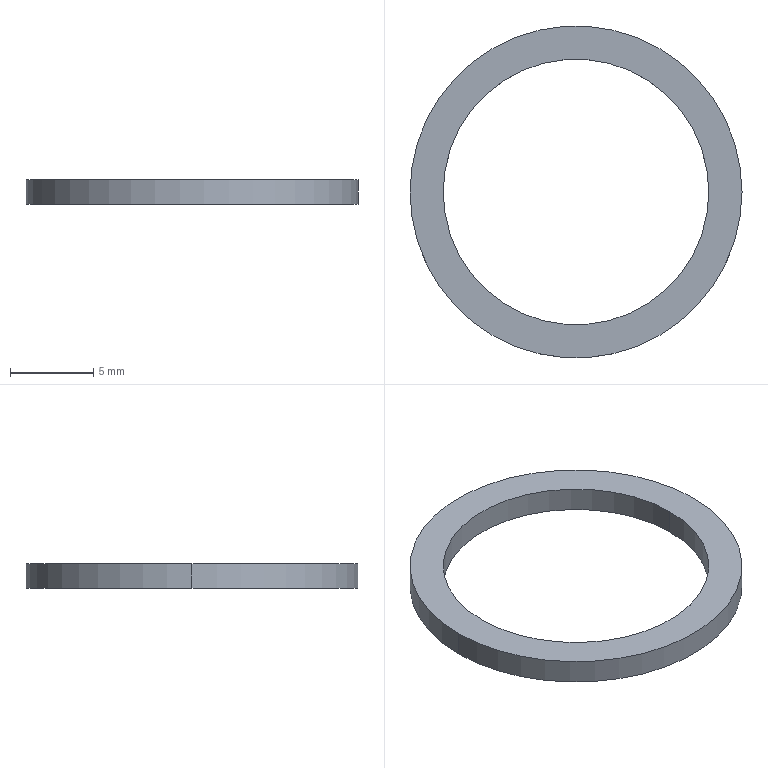Part | SolidWorks | features Extrusion 1 | 1 solid | 6 faces | box 20 x 20 x 1.5 mm | volume 169.646 mm3 | cylinder 4 | plane 2 | commonest cylinder face diameters 16 x2 20 x2
STEP:
#1=CARTESIAN_POINT('',(-8.,0.,1.5));
#2=VERTEX_POINT('',#1);
#3=CARTESIAN_POINT('',(8.,0.,1.5));
#4=VERTEX_POINT('',#3);
#5=CARTESIAN_POINT('',(0.,0.,1.5));
#6=DIRECTION('',(0.,0.,1.));
#7=DIRECTION('',(1.,0.,0.));
#8=AXIS2_PLACEMENT_3D('',#5,#6,#7);
#9=CIRCLE('',#8,8.);
#10=EDGE_CURVE('',#2,#4,#9,.T.);
#11=ORIENTED_EDGE('',*,*,#10,.T.);
#12=CARTESIAN_POINT('',(8.,0.,0.));
#13=VERTEX_POINT('',#12);
#14=CARTESIAN_POINT('',(8.,0.,1.5));
#15=DIRECTION('',(0.,0.,-1.));
#16=VECTOR('',#15,1000.);
#17=LINE('',#14,#16);
#18=EDGE_CURVE('',#4,#13,#17,.T.);
#19=ORIENTED_EDGE('',*,*,#18,.T.);
#20=CARTESIAN_POINT('',(-8.,0.,0.));
#21=VERTEX_POINT('',#20);
#22=CARTESIAN_POINT('',(0.,0.,0.));
#23=DIRECTION('',(0.,0.,1.));
#24=DIRECTION('',(1.,0.,0.));
#25=AXIS2_PLACEMENT_3D('',#22,#23,#24);
#26=CIRCLE('',#25,8.);
#27=EDGE_CURVE('',#21,#13,#26,.T.);
#28=ORIENTED_EDGE('',*,*,#27,.F.);
#29=CARTESIAN_POINT('',(-8.,0.,1.5));
#30=DIRECTION('',(0.,0.,-1.));
#31=VECTOR('',#30,1000.);
#32=LINE('',#29,#31);
#33=EDGE_CURVE('',#2,#21,#32,.T.);
#34=ORIENTED_EDGE('',*,*,#33,.F.);
#35=EDGE_LOOP('',(#11,#19,#28,#34));
#36=FACE_OUTER_BOUND('',#35,.T.);
#37=CARTESIAN_POINT('',(0.,0.,1.5));
#38=DIRECTION('',(0.,0.,-1.));
#39=DIRECTION('',(-1.,0.,0.));
#40=AXIS2_PLACEMENT_3D('',#37,#38,#39);
#41=CYLINDRICAL_SURFACE('',#40,8.);
#42=ADVANCED_FACE('',(#36),#41,.F.);
#43=CARTESIAN_POINT('',(10.,0.,1.5));
#44=VERTEX_POINT('',#43);
#45=CARTESIAN_POINT('',(-10.,0.,1.5));
#46=VERTEX_POINT('',#45);
#47=CARTESIAN_POINT('',(0.,0.,1.5));
#48=DIRECTION('',(0.,0.,1.));
#49=DIRECTION('',(1.,0.,0.));
#50=AXIS2_PLACEMENT_3D('',#47,#48,#49);
#51=CIRCLE('',#50,10.);
#52=EDGE_CURVE('',#44,#46,#51,.T.);
#53=ORIENTED_EDGE('',*,*,#52,.F.);
#54=CARTESIAN_POINT('',(10.,0.,0.));
#55=VERTEX_POINT('',#54);
#56=CARTESIAN_POINT('',(10.,0.,1.5));
#57=DIRECTION('',(0.,0.,-1.));
#58=VECTOR('',#57,1000.);
#59=LINE('',#56,#58);
#60=EDGE_CURVE('',#44,#55,#59,.T.);
#61=ORIENTED_EDGE('',*,*,#60,.T.);
#62=CARTESIAN_POINT('',(-10.,0.,0.));
#63=VERTEX_POINT('',#62);
#64=CARTESIAN_POINT('',(0.,0.,0.));
#65=DIRECTION('',(0.,0.,1.));
#66=DIRECTION('',(1.,0.,0.));
#67=AXIS2_PLACEMENT_3D('',#64,#65,#66);
#68=CIRCLE('',#67,10.);
#69=EDGE_CURVE('',#55,#63,#68,.T.);
#70=ORIENTED_EDGE('',*,*,#69,.T.);
#71=CARTESIAN_POINT('',(-10.,0.,1.5));
#72=DIRECTION('',(0.,0.,-1.));
#73=VECTOR('',#72,1000.);
#74=LINE('',#71,#73);
#75=EDGE_CURVE('',#46,#63,#74,.T.);
#76=ORIENTED_EDGE('',*,*,#75,.F.);
#77=EDGE_LOOP('',(#53,#61,#70,#76));
#78=FACE_OUTER_BOUND('',#77,.T.);
#79=CARTESIAN_POINT('',(0.,0.,1.5));
#80=DIRECTION('',(0.,0.,-1.));
#81=DIRECTION('',(-1.,0.,0.));
#82=AXIS2_PLACEMENT_3D('',#79,#80,#81);
#83=CYLINDRICAL_SURFACE('',#82,10.);
#84=ADVANCED_FACE('',(#78),#83,.T.);
#85=CARTESIAN_POINT('',(0.,0.,1.5));
#86=DIRECTION('',(0.,0.,1.));
#87=DIRECTION('',(1.,0.,0.));
#88=AXIS2_PLACEMENT_3D('',#85,#86,#87);
#89=CIRCLE('',#88,10.);
#90=EDGE_CURVE('',#46,#44,#89,.T.);
#91=ORIENTED_EDGE('',*,*,#90,.T.);
#92=ORIENTED_EDGE('',*,*,#52,.T.);
#93=EDGE_LOOP('',(#91,#92));
#94=FACE_OUTER_BOUND('',#93,.T.);
#95=ORIENTED_EDGE('',*,*,#10,.F.);
#96=CARTESIAN_POINT('',(0.,0.,1.5));
#97=DIRECTION('',(0.,0.,1.));
#98=DIRECTION('',(1.,0.,0.));
#99=AXIS2_PLACEMENT_3D('',#96,#97,#98);
#100=CIRCLE('',#99,8.);
#101=EDGE_CURVE('',#4,#2,#100,.T.);
#102=ORIENTED_EDGE('',*,*,#101,.F.);
#103=EDGE_LOOP('',(#95,#102));
#104=FACE_BOUND('',#103,.T.);
#105=CARTESIAN_POINT('',(0.,0.,1.5));
#106=DIRECTION('',(0.,0.,1.));
#107=DIRECTION('',(1.,0.,0.));
#108=AXIS2_PLACEMENT_3D('',#105,#106,#107);
#109=PLANE('',#108);
#110=ADVANCED_FACE('',(#94,#104),#109,.T.);
#111=CARTESIAN_POINT('',(0.,0.,0.));
#112=DIRECTION('',(0.,0.,1.));
#113=DIRECTION('',(1.,0.,0.));
#114=AXIS2_PLACEMENT_3D('',#111,#112,#113);
#115=CIRCLE('',#114,10.);
#116=EDGE_CURVE('',#63,#55,#115,.T.);
#117=ORIENTED_EDGE('',*,*,#116,.F.);
#118=ORIENTED_EDGE('',*,*,#69,.F.);
#119=EDGE_LOOP('',(#117,#118));
#120=FACE_OUTER_BOUND('',#119,.T.);
#121=ORIENTED_EDGE('',*,*,#27,.T.);
#122=CARTESIAN_POINT('',(0.,0.,0.));
#123=DIRECTION('',(0.,0.,1.));
#124=DIRECTION('',(1.,0.,0.));
#125=AXIS2_PLACEMENT_3D('',#122,#123,#124);
#126=CIRCLE('',#125,8.);
#127=EDGE_CURVE('',#13,#21,#126,.T.);
#128=ORIENTED_EDGE('',*,*,#127,.T.);
#129=EDGE_LOOP('',(#121,#128));
#130=FACE_BOUND('',#129,.T.);
#131=CARTESIAN_POINT('',(0.,0.,0.));
#132=DIRECTION('',(0.,0.,1.));
#133=DIRECTION('',(1.,0.,0.));
#134=AXIS2_PLACEMENT_3D('',#131,#132,#133);
#135=PLANE('',#134);
#136=ADVANCED_FACE('',(#120,#130),#135,.F.);
#137=ORIENTED_EDGE('',*,*,#60,.F.);
#138=ORIENTED_EDGE('',*,*,#90,.F.);
#139=ORIENTED_EDGE('',*,*,#75,.T.);
#140=ORIENTED_EDGE('',*,*,#116,.T.);
#141=EDGE_LOOP('',(#137,#138,#139,#140));
#142=FACE_OUTER_BOUND('',#141,.T.);
#143=CARTESIAN_POINT('',(0.,0.,1.5));
#144=DIRECTION('',(0.,0.,-1.));
#145=DIRECTION('',(-1.,0.,0.));
#146=AXIS2_PLACEMENT_3D('',#143,#144,#145);
#147=CYLINDRICAL_SURFACE('',#146,10.);
#148=ADVANCED_FACE('',(#142),#147,.T.);
#149=ORIENTED_EDGE('',*,*,#18,.F.);
#150=ORIENTED_EDGE('',*,*,#101,.T.);
#151=ORIENTED_EDGE('',*,*,#33,.T.);
#152=ORIENTED_EDGE('',*,*,#127,.F.);
#153=EDGE_LOOP('',(#149,#150,#151,#152));
#154=FACE_OUTER_BOUND('',#153,.T.);
#155=CARTESIAN_POINT('',(0.,0.,1.5));
#156=DIRECTION('',(0.,0.,-1.));
#157=DIRECTION('',(-1.,0.,0.));
#158=AXIS2_PLACEMENT_3D('',#155,#156,#157);
#159=CYLINDRICAL_SURFACE('',#158,8.);
#160=ADVANCED_FACE('',(#154),#159,.F.);
#161=CLOSED_SHELL('',(#42,#84,#110,#136,#148,#160));
#162=MANIFOLD_SOLID_BREP('',#161);
#163=CARTESIAN_POINT('',(0.,0.,0.));
#164=DIRECTION('',(0.,0.,1.));
#165=DIRECTION('',(1.,0.,0.));
#166=AXIS2_PLACEMENT_3D('',#163,#164,#165);
#167=(LENGTH_UNIT()NAMED_UNIT(*)SI_UNIT(.MILLI.,.METRE.));
#168=UNCERTAINTY_MEASURE_WITH_UNIT(LENGTH_MEASURE(0.00001),#167,'','');
#169=(NAMED_UNIT(*)PLANE_ANGLE_UNIT()SI_UNIT($,.RADIAN.));
#170=(NAMED_UNIT(*)SI_UNIT($,.STERADIAN.)SOLID_ANGLE_UNIT());
#171=(GEOMETRIC_REPRESENTATION_CONTEXT(3)GLOBAL_UNCERTAINTY_ASSIGNED_CONTEXT((#168))GLOBAL_UNIT_ASSIGNED_CONTEXT((#167,#169,#170))REPRESENTATION_CONTEXT('',''));
#172=ADVANCED_BREP_SHAPE_REPRESENTATION('',(#162,#166),#171);